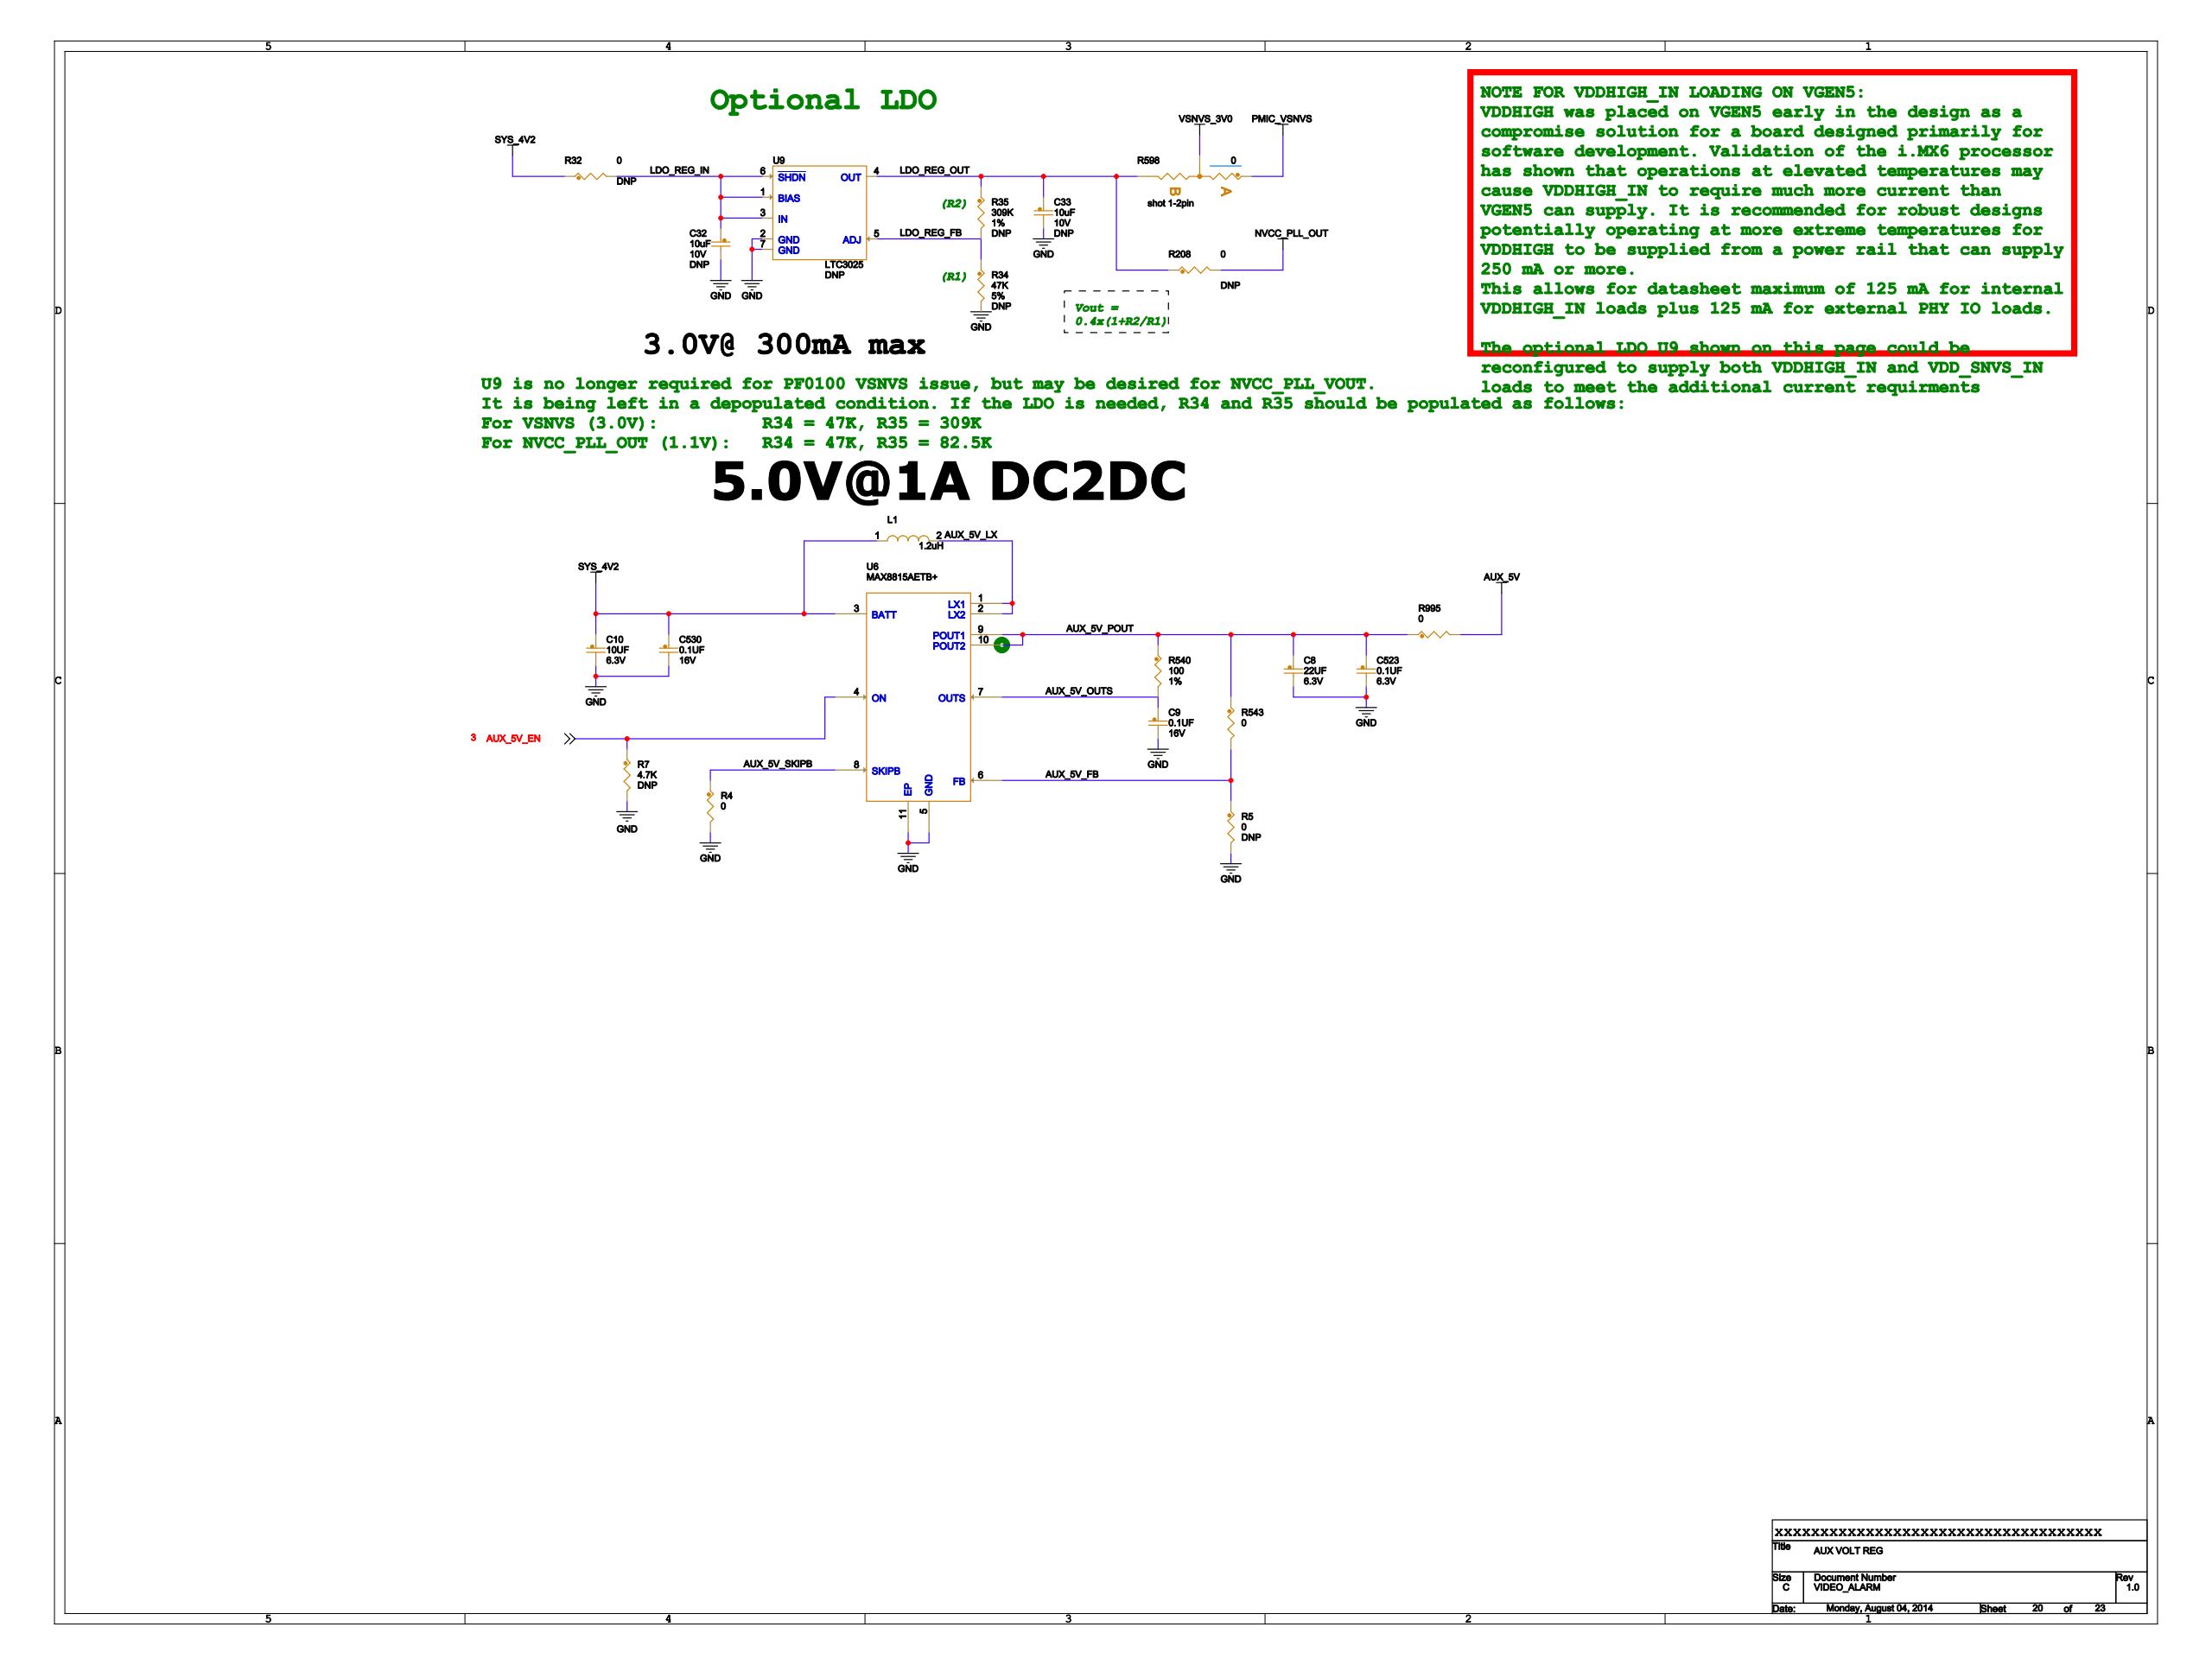Circuit board | Cadence Allegro | 994 parts | 728 nets | one sheet of the schematic
Parts on this sheet (reference | value | footprint):
C8 | 22UF | 0805_CC
C9 | 0.1UF | 0603_CC
C10 | 10UF | 0603_CC
C32 | 10uF | 0603_CC
C33 | 10uF | 0603_CC
C523 | 0.1UF | 0603_CC
C530 | 0.1UF | 0603_CC
L1 | 1.2uH | IND_VLCF4018
R4 | 0 | 0603_CC
R5 | 0 | 0603_CC
R7 | 4.7K | 0603_CC
R32 | 0 | 0805_CC
R34 | 47K | 0603_CC
R35 | 309K | 0603_CC
R208 | 0 | 0805_CC
R540 | 100 | 0603_CC
R543 | 0 | 0603_CC
R598 | 0 | R603-X2
R995 | 0 | 0805_CC
U6 | MAX8815AETB+ | TDFN10_0P5_3P1X3P1
U9 | LTC3025 | DFN6_2X2MM
Nets of these parts (net: part-pin ...):
GND: C8-2 C9-2 C10-2 C32-2 C33-2 C523-2 C530-2 R4-2 R5-2 R7-2 R34-2 U6-5 U6-11 U9-2 U9-7
SYS_4V2: C10-1 C530-1 L1-1 R32-1 U6-3
PMIC_VSNVS: R598-1
LDO_REG_OUT: C33-1 R35-1 R208-1 R598-3 U9-4
LDO_REG_FB: R34-1 R35-2 U9-5
AUX_5V_POUT: C8-1 C523-1 R540-1 R543-1 R995-1 U6-9 U6-10
AUX_5V_OUTS: C9-1 R540-2 U6-7
AUX_5V_FB: R5-1 R543-2 U6-6
AUX_5V_SKIPB: R4-1 U6-8
VSNVS_3V0: R598-2
AUX_5V: R995-2
LDO_REG_IN: C32-1 R32-2 U9-1 U9-3 U9-6
AUX_5V_LX: L1-2 U6-1 U6-2
AUX_5V_EN: R7-1 U6-4
NVCC_PLL_OUT: R208-2